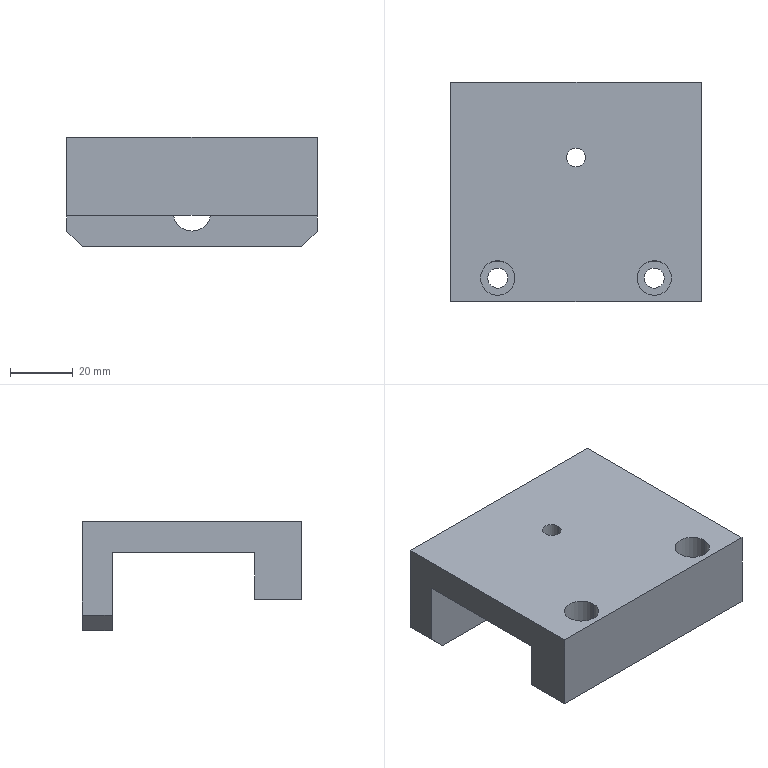Part | SolidWorks | features ICE 5, Chamfer 1, Extrusion 1, HoleWzd 1 | 1 solid | 26 faces | box 80 x 70 x 35 mm | volume 87735 mm3 | plane 14 | cylinder 12 | commonest cylinder face diameters 6.4 x4 11 x4 6 x2 12 x2
STEP:
#1=CARTESIAN_POINT('',(40.,60.5,7.));
#2=VERTEX_POINT('',#1);
#3=CARTESIAN_POINT('',(40.,60.5,-5.));
#4=VERTEX_POINT('',#3);
#5=CARTESIAN_POINT('',(40.,60.5,1.));
#6=DIRECTION('',(0.,-1.,0.));
#7=DIRECTION('',(0.,0.,1.));
#8=AXIS2_PLACEMENT_3D('',#5,#6,#7);
#9=CIRCLE('',#8,6.);
#10=EDGE_CURVE('',#2,#4,#9,.T.);
#11=ORIENTED_EDGE('',*,*,#10,.T.);
#12=CARTESIAN_POINT('',(40.,70.,-5.));
#13=VERTEX_POINT('',#12);
#14=CARTESIAN_POINT('',(40.,43.529,-5.));
#15=DIRECTION('',(0.,1.,0.));
#16=VECTOR('',#15,1000.);
#17=LINE('',#14,#16);
#18=EDGE_CURVE('',#4,#13,#17,.T.);
#19=ORIENTED_EDGE('',*,*,#18,.T.);
#20=CARTESIAN_POINT('',(40.,70.,7.));
#21=VERTEX_POINT('',#20);
#22=CARTESIAN_POINT('',(40.,70.,1.));
#23=DIRECTION('',(0.,1.,0.));
#24=DIRECTION('',(0.,0.,1.));
#25=AXIS2_PLACEMENT_3D('',#22,#23,#24);
#26=CIRCLE('',#25,6.);
#27=EDGE_CURVE('',#13,#21,#26,.T.);
#28=ORIENTED_EDGE('',*,*,#27,.T.);
#29=CARTESIAN_POINT('',(40.,43.529,7.));
#30=DIRECTION('',(0.,1.,0.));
#31=VECTOR('',#30,1000.);
#32=LINE('',#29,#31);
#33=EDGE_CURVE('',#2,#21,#32,.T.);
#34=ORIENTED_EDGE('',*,*,#33,.F.);
#35=EDGE_LOOP('',(#11,#19,#28,#34));
#36=FACE_OUTER_BOUND('',#35,.T.);
#37=CARTESIAN_POINT('',(40.,43.529,1.));
#38=DIRECTION('',(0.,1.,0.));
#39=DIRECTION('',(0.,0.,1.));
#40=AXIS2_PLACEMENT_3D('',#37,#38,#39);
#41=CYLINDRICAL_SURFACE('',#40,6.);
#42=ADVANCED_FACE('',(#36),#41,.F.);
#43=CARTESIAN_POINT('',(37.,46.,15.));
#44=VERTEX_POINT('',#43);
#45=CARTESIAN_POINT('',(43.,46.,15.));
#46=VERTEX_POINT('',#45);
#47=CARTESIAN_POINT('',(40.,46.,15.));
#48=DIRECTION('',(0.,0.,1.));
#49=DIRECTION('',(1.,0.,0.));
#50=AXIS2_PLACEMENT_3D('',#47,#48,#49);
#51=CIRCLE('',#50,3.);
#52=EDGE_CURVE('',#44,#46,#51,.T.);
#53=ORIENTED_EDGE('',*,*,#52,.F.);
#54=CARTESIAN_POINT('',(37.,46.,25.));
#55=VERTEX_POINT('',#54);
#56=CARTESIAN_POINT('',(37.,46.,15.));
#57=DIRECTION('',(0.,0.,1.));
#58=VECTOR('',#57,1000.);
#59=LINE('',#56,#58);
#60=EDGE_CURVE('',#44,#55,#59,.T.);
#61=ORIENTED_EDGE('',*,*,#60,.T.);
#62=CARTESIAN_POINT('',(43.,46.,25.));
#63=VERTEX_POINT('',#62);
#64=CARTESIAN_POINT('',(40.,46.,25.));
#65=DIRECTION('',(0.,0.,1.));
#66=DIRECTION('',(1.,0.,0.));
#67=AXIS2_PLACEMENT_3D('',#64,#65,#66);
#68=CIRCLE('',#67,3.);
#69=EDGE_CURVE('',#55,#63,#68,.T.);
#70=ORIENTED_EDGE('',*,*,#69,.T.);
#71=CARTESIAN_POINT('',(43.,46.,15.));
#72=DIRECTION('',(0.,0.,1.));
#73=VECTOR('',#72,1000.);
#74=LINE('',#71,#73);
#75=EDGE_CURVE('',#46,#63,#74,.T.);
#76=ORIENTED_EDGE('',*,*,#75,.F.);
#77=EDGE_LOOP('',(#53,#61,#70,#76));
#78=FACE_OUTER_BOUND('',#77,.T.);
#79=CARTESIAN_POINT('',(40.,46.,15.));
#80=DIRECTION('',(0.,0.,1.));
#81=DIRECTION('',(1.,0.,0.));
#82=AXIS2_PLACEMENT_3D('',#79,#80,#81);
#83=CYLINDRICAL_SURFACE('',#82,3.);
#84=ADVANCED_FACE('',(#78),#83,.F.);
#85=CARTESIAN_POINT('',(9.5,7.5,8.6));
#86=VERTEX_POINT('',#85);
#87=CARTESIAN_POINT('',(20.5,7.5,8.6));
#88=VERTEX_POINT('',#87);
#89=CARTESIAN_POINT('',(15.,7.5,8.6));
#90=DIRECTION('',(0.,0.,1.));
#91=DIRECTION('',(1.,0.,0.));
#92=AXIS2_PLACEMENT_3D('',#89,#90,#91);
#93=CIRCLE('',#92,5.5);
#94=EDGE_CURVE('',#86,#88,#93,.T.);
#95=ORIENTED_EDGE('',*,*,#94,.F.);
#96=CARTESIAN_POINT('',(9.5,7.5,25.));
#97=VERTEX_POINT('',#96);
#98=CARTESIAN_POINT('',(9.5,7.5,25.));
#99=DIRECTION('',(0.,0.,1.));
#100=VECTOR('',#99,1000.);
#101=LINE('',#98,#100);
#102=EDGE_CURVE('',#86,#97,#101,.T.);
#103=ORIENTED_EDGE('',*,*,#102,.T.);
#104=CARTESIAN_POINT('',(20.5,7.5,25.));
#105=VERTEX_POINT('',#104);
#106=CARTESIAN_POINT('',(15.,7.5,25.));
#107=DIRECTION('',(0.,0.,1.));
#108=DIRECTION('',(1.,0.,0.));
#109=AXIS2_PLACEMENT_3D('',#106,#107,#108);
#110=CIRCLE('',#109,5.5);
#111=EDGE_CURVE('',#97,#105,#110,.T.);
#112=ORIENTED_EDGE('',*,*,#111,.T.);
#113=CARTESIAN_POINT('',(20.5,7.5,25.));
#114=DIRECTION('',(0.,0.,1.));
#115=VECTOR('',#114,1000.);
#116=LINE('',#113,#115);
#117=EDGE_CURVE('',#88,#105,#116,.T.);
#118=ORIENTED_EDGE('',*,*,#117,.F.);
#119=EDGE_LOOP('',(#95,#103,#112,#118));
#120=FACE_OUTER_BOUND('',#119,.T.);
#121=CARTESIAN_POINT('',(15.,7.5,25.));
#122=DIRECTION('',(0.,0.,1.));
#123=DIRECTION('',(1.,0.,0.));
#124=AXIS2_PLACEMENT_3D('',#121,#122,#123);
#125=CYLINDRICAL_SURFACE('',#124,5.5);
#126=ADVANCED_FACE('',(#120),#125,.F.);
#127=CARTESIAN_POINT('',(59.5,7.5,8.6));
#128=VERTEX_POINT('',#127);
#129=CARTESIAN_POINT('',(70.5,7.5,8.6));
#130=VERTEX_POINT('',#129);
#131=CARTESIAN_POINT('',(65.,7.5,8.6));
#132=DIRECTION('',(0.,0.,1.));
#133=DIRECTION('',(1.,0.,0.));
#134=AXIS2_PLACEMENT_3D('',#131,#132,#133);
#135=CIRCLE('',#134,5.5);
#136=EDGE_CURVE('',#128,#130,#135,.T.);
#137=ORIENTED_EDGE('',*,*,#136,.F.);
#138=CARTESIAN_POINT('',(59.5,7.5,25.));
#139=VERTEX_POINT('',#138);
#140=CARTESIAN_POINT('',(59.5,7.5,25.));
#141=DIRECTION('',(0.,0.,1.));
#142=VECTOR('',#141,1000.);
#143=LINE('',#140,#142);
#144=EDGE_CURVE('',#128,#139,#143,.T.);
#145=ORIENTED_EDGE('',*,*,#144,.T.);
#146=CARTESIAN_POINT('',(70.5,7.5,25.));
#147=VERTEX_POINT('',#146);
#148=CARTESIAN_POINT('',(65.,7.5,25.));
#149=DIRECTION('',(0.,0.,1.));
#150=DIRECTION('',(1.,0.,0.));
#151=AXIS2_PLACEMENT_3D('',#148,#149,#150);
#152=CIRCLE('',#151,5.5);
#153=EDGE_CURVE('',#139,#147,#152,.T.);
#154=ORIENTED_EDGE('',*,*,#153,.T.);
#155=CARTESIAN_POINT('',(70.5,7.5,25.));
#156=DIRECTION('',(0.,0.,1.));
#157=VECTOR('',#156,1000.);
#158=LINE('',#155,#157);
#159=EDGE_CURVE('',#130,#147,#158,.T.);
#160=ORIENTED_EDGE('',*,*,#159,.F.);
#161=EDGE_LOOP('',(#137,#145,#154,#160));
#162=FACE_OUTER_BOUND('',#161,.T.);
#163=CARTESIAN_POINT('',(65.,7.5,25.));
#164=DIRECTION('',(0.,0.,1.));
#165=DIRECTION('',(1.,0.,0.));
#166=AXIS2_PLACEMENT_3D('',#163,#164,#165);
#167=CYLINDRICAL_SURFACE('',#166,5.5);
#168=ADVANCED_FACE('',(#162),#167,.F.);
#169=CARTESIAN_POINT('',(11.8,7.5,0.));
#170=VERTEX_POINT('',#169);
#171=CARTESIAN_POINT('',(18.2,7.5,0.));
#172=VERTEX_POINT('',#171);
#173=CARTESIAN_POINT('',(15.,7.5,0.));
#174=DIRECTION('',(0.,0.,1.));
#175=DIRECTION('',(1.,0.,0.));
#176=AXIS2_PLACEMENT_3D('',#173,#174,#175);
#177=CIRCLE('',#176,3.2);
#178=EDGE_CURVE('',#170,#172,#177,.T.);
#179=ORIENTED_EDGE('',*,*,#178,.F.);
#180=CARTESIAN_POINT('',(11.8,7.5,8.6));
#181=VERTEX_POINT('',#180);
#182=CARTESIAN_POINT('',(11.8,7.5,25.));
#183=DIRECTION('',(0.,0.,1.));
#184=VECTOR('',#183,1000.);
#185=LINE('',#182,#184);
#186=EDGE_CURVE('',#170,#181,#185,.T.);
#187=ORIENTED_EDGE('',*,*,#186,.T.);
#188=CARTESIAN_POINT('',(18.2,7.5,8.6));
#189=VERTEX_POINT('',#188);
#190=CARTESIAN_POINT('',(15.,7.5,8.6));
#191=DIRECTION('',(0.,0.,-1.));
#192=DIRECTION('',(1.,0.,0.));
#193=AXIS2_PLACEMENT_3D('',#190,#191,#192);
#194=CIRCLE('',#193,3.2);
#195=EDGE_CURVE('',#189,#181,#194,.T.);
#196=ORIENTED_EDGE('',*,*,#195,.F.);
#197=CARTESIAN_POINT('',(18.2,7.5,25.));
#198=DIRECTION('',(0.,0.,1.));
#199=VECTOR('',#198,1000.);
#200=LINE('',#197,#199);
#201=EDGE_CURVE('',#172,#189,#200,.T.);
#202=ORIENTED_EDGE('',*,*,#201,.F.);
#203=EDGE_LOOP('',(#179,#187,#196,#202));
#204=FACE_OUTER_BOUND('',#203,.T.);
#205=CARTESIAN_POINT('',(15.,7.5,25.));
#206=DIRECTION('',(0.,0.,1.));
#207=DIRECTION('',(1.,0.,0.));
#208=AXIS2_PLACEMENT_3D('',#205,#206,#207);
#209=CYLINDRICAL_SURFACE('',#208,3.2);
#210=ADVANCED_FACE('',(#204),#209,.F.);
#211=CARTESIAN_POINT('',(61.8,7.5,0.));
#212=VERTEX_POINT('',#211);
#213=CARTESIAN_POINT('',(68.2,7.5,0.));
#214=VERTEX_POINT('',#213);
#215=CARTESIAN_POINT('',(65.,7.5,0.));
#216=DIRECTION('',(0.,0.,1.));
#217=DIRECTION('',(1.,0.,0.));
#218=AXIS2_PLACEMENT_3D('',#215,#216,#217);
#219=CIRCLE('',#218,3.2);
#220=EDGE_CURVE('',#212,#214,#219,.T.);
#221=ORIENTED_EDGE('',*,*,#220,.F.);
#222=CARTESIAN_POINT('',(61.8,7.5,8.6));
#223=VERTEX_POINT('',#222);
#224=CARTESIAN_POINT('',(61.8,7.5,25.));
#225=DIRECTION('',(0.,0.,1.));
#226=VECTOR('',#225,1000.);
#227=LINE('',#224,#226);
#228=EDGE_CURVE('',#212,#223,#227,.T.);
#229=ORIENTED_EDGE('',*,*,#228,.T.);
#230=CARTESIAN_POINT('',(68.2,7.5,8.6));
#231=VERTEX_POINT('',#230);
#232=CARTESIAN_POINT('',(65.,7.5,8.6));
#233=DIRECTION('',(0.,0.,-1.));
#234=DIRECTION('',(1.,0.,0.));
#235=AXIS2_PLACEMENT_3D('',#232,#233,#234);
#236=CIRCLE('',#235,3.2);
#237=EDGE_CURVE('',#231,#223,#236,.T.);
#238=ORIENTED_EDGE('',*,*,#237,.F.);
#239=CARTESIAN_POINT('',(68.2,7.5,25.));
#240=DIRECTION('',(0.,0.,1.));
#241=VECTOR('',#240,1000.);
#242=LINE('',#239,#241);
#243=EDGE_CURVE('',#214,#231,#242,.T.);
#244=ORIENTED_EDGE('',*,*,#243,.F.);
#245=EDGE_LOOP('',(#221,#229,#238,#244));
#246=FACE_OUTER_BOUND('',#245,.T.);
#247=CARTESIAN_POINT('',(65.,7.5,25.));
#248=DIRECTION('',(0.,0.,1.));
#249=DIRECTION('',(1.,0.,0.));
#250=AXIS2_PLACEMENT_3D('',#247,#248,#249);
#251=CYLINDRICAL_SURFACE('',#250,3.2);
#252=ADVANCED_FACE('',(#246),#251,.F.);
#253=ORIENTED_EDGE('',*,*,#228,.F.);
#254=CARTESIAN_POINT('',(65.,7.5,0.));
#255=DIRECTION('',(0.,0.,1.));
#256=DIRECTION('',(1.,0.,0.));
#257=AXIS2_PLACEMENT_3D('',#254,#255,#256);
#258=CIRCLE('',#257,3.2);
#259=EDGE_CURVE('',#214,#212,#258,.T.);
#260=ORIENTED_EDGE('',*,*,#259,.F.);
#261=ORIENTED_EDGE('',*,*,#243,.T.);
#262=CARTESIAN_POINT('',(65.,7.5,8.6));
#263=DIRECTION('',(0.,0.,-1.));
#264=DIRECTION('',(1.,0.,0.));
#265=AXIS2_PLACEMENT_3D('',#262,#263,#264);
#266=CIRCLE('',#265,3.2);
#267=EDGE_CURVE('',#223,#231,#266,.T.);
#268=ORIENTED_EDGE('',*,*,#267,.F.);
#269=EDGE_LOOP('',(#253,#260,#261,#268));
#270=FACE_OUTER_BOUND('',#269,.T.);
#271=CARTESIAN_POINT('',(65.,7.5,25.));
#272=DIRECTION('',(0.,0.,1.));
#273=DIRECTION('',(1.,0.,0.));
#274=AXIS2_PLACEMENT_3D('',#271,#272,#273);
#275=CYLINDRICAL_SURFACE('',#274,3.2);
#276=ADVANCED_FACE('',(#270),#275,.F.);
#277=ORIENTED_EDGE('',*,*,#186,.F.);
#278=CARTESIAN_POINT('',(15.,7.5,0.));
#279=DIRECTION('',(0.,0.,1.));
#280=DIRECTION('',(1.,0.,0.));
#281=AXIS2_PLACEMENT_3D('',#278,#279,#280);
#282=CIRCLE('',#281,3.2);
#283=EDGE_CURVE('',#172,#170,#282,.T.);
#284=ORIENTED_EDGE('',*,*,#283,.F.);
#285=ORIENTED_EDGE('',*,*,#201,.T.);
#286=CARTESIAN_POINT('',(15.,7.5,8.6));
#287=DIRECTION('',(0.,0.,-1.));
#288=DIRECTION('',(1.,0.,0.));
#289=AXIS2_PLACEMENT_3D('',#286,#287,#288);
#290=CIRCLE('',#289,3.2);
#291=EDGE_CURVE('',#181,#189,#290,.T.);
#292=ORIENTED_EDGE('',*,*,#291,.F.);
#293=EDGE_LOOP('',(#277,#284,#285,#292));
#294=FACE_OUTER_BOUND('',#293,.T.);
#295=CARTESIAN_POINT('',(15.,7.5,25.));
#296=DIRECTION('',(0.,0.,1.));
#297=DIRECTION('',(1.,0.,0.));
#298=AXIS2_PLACEMENT_3D('',#295,#296,#297);
#299=CYLINDRICAL_SURFACE('',#298,3.2);
#300=ADVANCED_FACE('',(#294),#299,.F.);
#301=CARTESIAN_POINT('',(0.,70.,25.));
#302=VERTEX_POINT('',#301);
#303=CARTESIAN_POINT('',(0.,70.,-5.));
#304=VERTEX_POINT('',#303);
#305=CARTESIAN_POINT('',(0.,70.,25.));
#306=DIRECTION('',(0.,0.,-1.));
#307=VECTOR('',#306,1000.);
#308=LINE('',#305,#307);
#309=EDGE_CURVE('',#302,#304,#308,.T.);
#310=ORIENTED_EDGE('',*,*,#309,.T.);
#311=CARTESIAN_POINT('',(0.,60.5,-5.));
#312=VERTEX_POINT('',#311);
#313=CARTESIAN_POINT('',(0.,60.5,-5.));
#314=DIRECTION('',(0.,-1.,0.));
#315=VECTOR('',#314,1000.);
#316=LINE('',#313,#315);
#317=EDGE_CURVE('',#304,#312,#316,.T.);
#318=ORIENTED_EDGE('',*,*,#317,.T.);
#319=CARTESIAN_POINT('',(0.,60.5,15.));
#320=VERTEX_POINT('',#319);
#321=CARTESIAN_POINT('',(0.,60.5,25.));
#322=DIRECTION('',(0.,0.,1.));
#323=VECTOR('',#322,1000.);
#324=LINE('',#321,#323);
#325=EDGE_CURVE('',#312,#320,#324,.T.);
#326=ORIENTED_EDGE('',*,*,#325,.T.);
#327=CARTESIAN_POINT('',(0.,15.,15.));
#328=VERTEX_POINT('',#327);
#329=CARTESIAN_POINT('',(0.,0.,15.));
#330=DIRECTION('',(0.,-1.,0.));
#331=VECTOR('',#330,1000.);
#332=LINE('',#329,#331);
#333=EDGE_CURVE('',#320,#328,#332,.T.);
#334=ORIENTED_EDGE('',*,*,#333,.T.);
#335=CARTESIAN_POINT('',(0.,15.,0.));
#336=VERTEX_POINT('',#335);
#337=CARTESIAN_POINT('',(0.,15.,25.));
#338=DIRECTION('',(0.,0.,-1.));
#339=VECTOR('',#338,1000.);
#340=LINE('',#337,#339);
#341=EDGE_CURVE('',#328,#336,#340,.T.);
#342=ORIENTED_EDGE('',*,*,#341,.T.);
#343=CARTESIAN_POINT('',(0.,0.,0.));
#344=VERTEX_POINT('',#343);
#345=CARTESIAN_POINT('',(0.,0.,0.));
#346=DIRECTION('',(0.,-1.,0.));
#347=VECTOR('',#346,1000.);
#348=LINE('',#345,#347);
#349=EDGE_CURVE('',#336,#344,#348,.T.);
#350=ORIENTED_EDGE('',*,*,#349,.T.);
#351=CARTESIAN_POINT('',(0.,0.,25.));
#352=VERTEX_POINT('',#351);
#353=CARTESIAN_POINT('',(0.,0.,25.));
#354=DIRECTION('',(0.,0.,-1.));
#355=VECTOR('',#354,1000.);
#356=LINE('',#353,#355);
#357=EDGE_CURVE('',#352,#344,#356,.T.);
#358=ORIENTED_EDGE('',*,*,#357,.F.);
#359=CARTESIAN_POINT('',(0.,0.,25.));
#360=DIRECTION('',(0.,-1.,0.));
#361=VECTOR('',#360,1000.);
#362=LINE('',#359,#361);
#363=EDGE_CURVE('',#302,#352,#362,.T.);
#364=ORIENTED_EDGE('',*,*,#363,.F.);
#365=EDGE_LOOP('',(#310,#318,#326,#334,#342,#350,#358,#364));
#366=FACE_OUTER_BOUND('',#365,.T.);
#367=CARTESIAN_POINT('',(0.,0.,25.));
#368=DIRECTION('',(1.,0.,0.));
#369=DIRECTION('',(0.,1.,0.));
#370=AXIS2_PLACEMENT_3D('',#367,#368,#369);
#371=PLANE('',#370);
#372=ADVANCED_FACE('',(#366),#371,.F.);
#373=CARTESIAN_POINT('',(80.,0.,0.));
#374=VERTEX_POINT('',#373);
#375=CARTESIAN_POINT('',(0.,0.,0.));
#376=DIRECTION('',(1.,0.,0.));
#377=VECTOR('',#376,1000.);
#378=LINE('',#375,#377);
#379=EDGE_CURVE('',#344,#374,#378,.T.);
#380=ORIENTED_EDGE('',*,*,#379,.T.);
#381=CARTESIAN_POINT('',(80.,0.,25.));
#382=VERTEX_POINT('',#381);
#383=CARTESIAN_POINT('',(80.,0.,25.));
#384=DIRECTION('',(0.,0.,-1.));
#385=VECTOR('',#384,1000.);
#386=LINE('',#383,#385);
#387=EDGE_CURVE('',#382,#374,#386,.T.);
#388=ORIENTED_EDGE('',*,*,#387,.F.);
#389=CARTESIAN_POINT('',(0.,0.,25.));
#390=DIRECTION('',(1.,0.,0.));
#391=VECTOR('',#390,1000.);
#392=LINE('',#389,#391);
#393=EDGE_CURVE('',#352,#382,#392,.T.);
#394=ORIENTED_EDGE('',*,*,#393,.F.);
#395=ORIENTED_EDGE('',*,*,#357,.T.);
#396=EDGE_LOOP('',(#380,#388,#394,#395));
#397=FACE_OUTER_BOUND('',#396,.T.);
#398=CARTESIAN_POINT('',(0.,0.,25.));
#399=DIRECTION('',(0.,1.,0.));
#400=DIRECTION('',(0.,0.,1.));
#401=AXIS2_PLACEMENT_3D('',#398,#399,#400);
#402=PLANE('',#401);
#403=ADVANCED_FACE('',(#397),#402,.F.);
#404=CARTESIAN_POINT('',(80.,60.5,-5.));
#405=VERTEX_POINT('',#404);
#406=CARTESIAN_POINT('',(80.,60.5,15.));
#407=VERTEX_POINT('',#406);
#408=CARTESIAN_POINT('',(80.,60.5,15.));
#409=DIRECTION('',(0.,0.,1.));
#410=VECTOR('',#409,1000.);
#411=LINE('',#408,#410);
#412=EDGE_CURVE('',#405,#407,#411,.T.);
#413=ORIENTED_EDGE('',*,*,#412,.F.);
#414=CARTESIAN_POINT('',(80.,70.,-5.));
#415=VERTEX_POINT('',#414);
#416=CARTESIAN_POINT('',(80.,70.,-5.));
#417=DIRECTION('',(0.,1.,0.));
#418=VECTOR('',#417,1000.);
#419=LINE('',#416,#418);
#420=EDGE_CURVE('',#405,#415,#419,.T.);
#421=ORIENTED_EDGE('',*,*,#420,.T.);
#422=CARTESIAN_POINT('',(80.,70.,25.));
#423=VERTEX_POINT('',#422);
#424=CARTESIAN_POINT('',(80.,70.,25.));
#425=DIRECTION('',(0.,0.,-1.));
#426=VECTOR('',#425,1000.);
#427=LINE('',#424,#426);
#428=EDGE_CURVE('',#423,#415,#427,.T.);
#429=ORIENTED_EDGE('',*,*,#428,.F.);
#430=CARTESIAN_POINT('',(80.,0.,25.));
#431=DIRECTION('',(0.,1.,0.));
#432=VECTOR('',#431,1000.);
#433=LINE('',#430,#432);
#434=EDGE_CURVE('',#382,#423,#433,.T.);
#435=ORIENTED_EDGE('',*,*,#434,.F.);
#436=ORIENTED_EDGE('',*,*,#387,.T.);
#437=CARTESIAN_POINT('',(80.,15.,0.));
#438=VERTEX_POINT('',#437);
#439=CARTESIAN_POINT('',(80.,0.,0.));
#440=DIRECTION('',(0.,1.,0.));
#441=VECTOR('',#440,1000.);
#442=LINE('',#439,#441);
#443=EDGE_CURVE('',#374,#438,#442,.T.);
#444=ORIENTED_EDGE('',*,*,#443,.T.);
#445=CARTESIAN_POINT('',(80.,15.,15.));
#446=VERTEX_POINT('',#445);
#447=CARTESIAN_POINT('',(80.,15.,15.));
#448=DIRECTION('',(0.,0.,-1.));
#449=VECTOR('',#448,1000.);
#450=LINE('',#447,#449);
#451=EDGE_CURVE('',#446,#438,#450,.T.);
#452=ORIENTED_EDGE('',*,*,#451,.F.);
#453=CARTESIAN_POINT('',(80.,60.5,15.));
#454=DIRECTION('',(0.,-1.,0.));
#455=VECTOR('',#454,1000.);
#456=LINE('',#453,#455);
#457=EDGE_CURVE('',#407,#446,#456,.T.);
#458=ORIENTED_EDGE('',*,*,#457,.F.);
#459=EDGE_LOOP('',(#413,#421,#429,#435,#436,#444,#452,#458));
#460=FACE_OUTER_BOUND('',#459,.T.);
#461=CARTESIAN_POINT('',(80.,0.,25.));
#462=DIRECTION('',(-1.,0.,0.));
#463=DIRECTION('',(0.,-1.,0.));
#464=AXIS2_PLACEMENT_3D('',#461,#462,#463);
#465=PLANE('',#464);
#466=ADVANCED_FACE('',(#460),#465,.F.);
#467=CARTESIAN_POINT('',(40.,70.,1.));
#468=DIRECTION('',(0.,1.,0.));
#469=DIRECTION('',(0.,0.,1.));
#470=AXIS2_PLACEMENT_3D('',#467,#468,#469);
#471=CIRCLE('',#470,6.);
#472=EDGE_CURVE('',#21,#13,#471,.T.);
#473=ORIENTED_EDGE('',*,*,#472,.F.);
#474=ORIENTED_EDGE('',*,*,#27,.F.);
#475=EDGE_LOOP('',(#473,#474));
#476=FACE_BOUND('',#475,.T.);
#477=CARTESIAN_POINT('',(5.,70.,-10.));
#478=VERTEX_POINT('',#477);
#479=CARTESIAN_POINT('',(75.,70.,-10.));
#480=VERTEX_POINT('',#479);
#481=CARTESIAN_POINT('',(0.,70.,-10.));
#482=DIRECTION('',(1.,0.,0.));
#483=VECTOR('',#482,1000.);
#484=LINE('',#481,#483);
#485=EDGE_CURVE('',#478,#480,#484,.T.);
#486=ORIENTED_EDGE('',*,*,#485,.F.);
#487=CARTESIAN_POINT('',(5.,70.,-10.));
#488=DIRECTION('',(-0.7071,0.,0.7071));
#489=VECTOR('',#488,1000.);
#490=LINE('',#487,#489);
#491=EDGE_CURVE('',#478,#304,#490,.T.);
#492=ORIENTED_EDGE('',*,*,#491,.T.);
#493=ORIENTED_EDGE('',*,*,#309,.F.);
#494=CARTESIAN_POINT('',(0.,70.,25.));
#495=DIRECTION('',(-1.,0.,0.));
#496=VECTOR('',#495,1000.);
#497=LINE('',#494,#496);
#498=EDGE_CURVE('',#423,#302,#497,.T.);
#499=ORIENTED_EDGE('',*,*,#498,.F.);
#500=ORIENTED_EDGE('',*,*,#428,.T.);
#501=CARTESIAN_POINT('',(75.,70.,-10.));
#502=DIRECTION('',(-0.7071,0.,-0.7071));
#503=VECTOR('',#502,1000.);
#504=LINE('',#501,#503);
#505=EDGE_CURVE('',#415,#480,#504,.T.);
#506=ORIENTED_EDGE('',*,*,#505,.T.);
#507=EDGE_LOOP('',(#486,#492,#493,#499,#500,#506));
#508=FACE_OUTER_BOUND('',#507,.T.);
#509=CARTESIAN_POINT('',(0.,70.,25.));
#510=DIRECTION('',(0.,-1.,0.));
#511=DIRECTION('',(0.,0.,-1.));
#512=AXIS2_PLACEMENT_3D('',#509,#510,#511);
#513=PLANE('',#512);
#514=ADVANCED_FACE('',(#476,#508),#513,.F.);
#515=CARTESIAN_POINT('',(40.,46.,25.));
#516=DIRECTION('',(0.,0.,1.));
#517=DIRECTION('',(1.,0.,0.));
#518=AXIS2_PLACEMENT_3D('',#515,#516,#517);
#519=CIRCLE('',#518,3.);
#520=EDGE_CURVE('',#63,#55,#519,.T.);
#521=ORIENTED_EDGE('',*,*,#520,.F.);
#522=ORIENTED_EDGE('',*,*,#69,.F.);
#523=EDGE_LOOP('',(#521,#522));
#524=FACE_BOUND('',#523,.T.);
#525=CARTESIAN_POINT('',(15.,7.5,25.));
#526=DIRECTION('',(0.,0.,1.));
#527=DIRECTION('',(1.,0.,0.));
#528=AXIS2_PLACEMENT_3D('',#525,#526,#527);
#529=CIRCLE('',#528,5.5);
#530=EDGE_CURVE('',#105,#97,#529,.T.);
#531=ORIENTED_EDGE('',*,*,#530,.F.);
#532=ORIENTED_EDGE('',*,*,#111,.F.);
#533=EDGE_LOOP('',(#531,#532));
#534=FACE_BOUND('',#533,.T.);
#535=CARTESIAN_POINT('',(65.,7.5,25.));
#536=DIRECTION('',(0.,0.,1.));
#537=DIRECTION('',(1.,0.,0.));
#538=AXIS2_PLACEMENT_3D('',#535,#536,#537);
#539=CIRCLE('',#538,5.5);
#540=EDGE_CURVE('',#147,#139,#539,.T.);
#541=ORIENTED_EDGE('',*,*,#540,.F.);
#542=ORIENTED_EDGE('',*,*,#153,.F.);
#543=EDGE_LOOP('',(#541,#542));
#544=FACE_BOUND('',#543,.T.);
#545=ORIENTED_EDGE('',*,*,#363,.T.);
#546=ORIENTED_EDGE('',*,*,#393,.T.);
#547=ORIENTED_EDGE('',*,*,#434,.T.);
#548=ORIENTED_EDGE('',*,*,#498,.T.);
#549=EDGE_LOOP('',(#545,#546,#547,#548));
#550=FACE_OUTER_BOUND('',#549,.T.);
#551=CARTESIAN_POINT('',(0.,0.,25.));
#552=DIRECTION('',(0.,0.,-1.));
#553=DIRECTION('',(-1.,0.,0.));
#554=AXIS2_PLACEMENT_3D('',#551,#552,#553);
#555=PLANE('',#554);
#556=ADVANCED_FACE('',(#524,#534,#544,#550),#555,.F.);
#557=ORIENTED_EDGE('',*,*,#283,.T.);
#558=ORIENTED_EDGE('',*,*,#178,.T.);
#559=EDGE_LOOP('',(#557,#558));
#560=FACE_BOUND('',#559,.T.);
#561=ORIENTED_EDGE('',*,*,#259,.T.);
#562=ORIENTED_EDGE('',*,*,#220,.T.);
#563=EDGE_LOOP('',(#561,#562));
#564=FACE_BOUND('',#563,.T.);
#565=CARTESIAN_POINT('',(0.,15.,0.));
#566=DIRECTION('',(-1.,0.,0.));
#567=VECTOR('',#566,1000.);
#568=LINE('',#565,#567);
#569=EDGE_CURVE('',#438,#336,#568,.T.);
#570=ORIENTED_EDGE('',*,*,#569,.F.);
#571=ORIENTED_EDGE('',*,*,#443,.F.);
#572=ORIENTED_EDGE('',*,*,#379,.F.);
#573=ORIENTED_EDGE('',*,*,#349,.F.);
#574=EDGE_LOOP('',(#570,#571,#572,#573));
#575=FACE_OUTER_BOUND('',#574,.T.);
#576=CARTESIAN_POINT('',(0.,0.,0.));
#577=DIRECTION('',(0.,0.,-1.));
#578=DIRECTION('',(-1.,0.,0.));
#579=AXIS2_PLACEMENT_3D('',#576,#577,#578);
#580=PLANE('',#579);
#581=ADVANCED_FACE('',(#560,#564,#575),#580,.T.);
#582=CARTESIAN_POINT('',(40.,46.,15.));
#583=DIRECTION('',(0.,0.,1.));
#584=DIRECTION('',(1.,0.,0.));
#585=AXIS2_PLACEMENT_3D('',#582,#583,#584);
#586=CIRCLE('',#585,3.);
#587=EDGE_CURVE('',#46,#44,#586,.T.);
#588=ORIENTED_EDGE('',*,*,#587,.T.);
#589=ORIENTED_EDGE('',*,*,#52,.T.);
#590=EDGE_LOOP('',(#588,#589));
#591=FACE_BOUND('',#590,.T.);
#592=CARTESIAN_POINT('',(-29.,60.5,15.));
#593=DIRECTION('',(1.,0.,0.));
#594=VECTOR('',#593,1000.);
#595=LINE('',#592,#594);
#596=EDGE_CURVE('',#320,#407,#595,.T.);
#597=ORIENTED_EDGE('',*,*,#596,.T.);
#598=ORIENTED_EDGE('',*,*,#457,.T.);
#599=CARTESIAN_POINT('',(-29.,15.,15.));
#600=DIRECTION('',(1.,0.,0.));
#601=VECTOR('',#600,1000.);
#602=LINE('',#599,#601);
#603=EDGE_CURVE('',#328,#446,#602,.T.);
#604=ORIENTED_EDGE('',*,*,#603,.F.);
#605=ORIENTED_EDGE('',*,*,#333,.F.);
#606=EDGE_LOOP('',(#597,#598,#604,#605));
#607=FACE_OUTER_BOUND('',#606,.T.);
#608=CARTESIAN_POINT('',(-29.,60.5,15.));
#609=DIRECTION('',(0.,0.,1.));
#610=DIRECTION('',(0.,-1.,0.));
#611=AXIS2_PLACEMENT_3D('',#608,#609,#610);
#612=PLANE('',#611);
#613=ADVANCED_FACE('',(#591,#607),#612,.F.);
#614=ORIENTED_EDGE('',*,*,#10,.F.);
#615=CARTESIAN_POINT('',(40.,60.5,1.));
#616=DIRECTION('',(0.,-1.,0.));
#617=DIRECTION('',(0.,0.,1.));
#618=AXIS2_PLACEMENT_3D('',#615,#616,#617);
#619=CIRCLE('',#618,6.);
#620=EDGE_CURVE('',#4,#2,#619,.T.);
#621=ORIENTED_EDGE('',*,*,#620,.F.);
#622=EDGE_LOOP('',(#614,#621));
#623=FACE_BOUND('',#622,.T.);
#624=ORIENTED_EDGE('',*,*,#325,.F.);
#625=CARTESIAN_POINT('',(5.,60.5,-10.));
#626=VERTEX_POINT('',#625);
#627=CARTESIAN_POINT('',(5.,60.5,-10.));
#628=DIRECTION('',(0.7071,0.,-0.7071));
#629=VECTOR('',#628,1000.);
#630=LINE('',#627,#629);
#631=EDGE_CURVE('',#312,#626,#630,.T.);
#632=ORIENTED_EDGE('',*,*,#631,.T.);
#633=CARTESIAN_POINT('',(75.,60.5,-10.));
#634=VERTEX_POINT('',#633);
#635=CARTESIAN_POINT('',(80.,60.5,-10.));
#636=DIRECTION('',(-1.,0.,0.));
#637=VECTOR('',#636,1000.);
#638=LINE('',#635,#637);
#639=EDGE_CURVE('',#634,#626,#638,.T.);
#640=ORIENTED_EDGE('',*,*,#639,.F.);
#641=CARTESIAN_POINT('',(75.,60.5,-10.));
#642=DIRECTION('',(0.7071,0.,0.7071));
#643=VECTOR('',#642,1000.);
#644=LINE('',#641,#643);
#645=EDGE_CURVE('',#634,#405,#644,.T.);
#646=ORIENTED_EDGE('',*,*,#645,.T.);
#647=ORIENTED_EDGE('',*,*,#412,.T.);
#648=ORIENTED_EDGE('',*,*,#596,.F.);
#649=EDGE_LOOP('',(#624,#632,#640,#646,#647,#648));
#650=FACE_OUTER_BOUND('',#649,.T.);
#651=CARTESIAN_POINT('',(-29.,60.5,15.));
#652=DIRECTION('',(0.,1.,0.));
#653=DIRECTION('',(0.,0.,1.));
#654=AXIS2_PLACEMENT_3D('',#651,#652,#653);
#655=PLANE('',#654);
#656=ADVANCED_FACE('',(#623,#650),#655,.F.);
#657=ORIENTED_EDGE('',*,*,#603,.T.);
#658=ORIENTED_EDGE('',*,*,#451,.T.);
#659=ORIENTED_EDGE('',*,*,#569,.T.);
#660=ORIENTED_EDGE('',*,*,#341,.F.);
#661=EDGE_LOOP('',(#657,#658,#659,#660));
#662=FACE_OUTER_BOUND('',#661,.T.);
#663=CARTESIAN_POINT('',(-29.,15.,15.));
#664=DIRECTION('',(0.,-1.,0.));
#665=DIRECTION('',(0.,0.,-1.));
#666=AXIS2_PLACEMENT_3D('',#663,#664,#665);
#667=PLANE('',#666);
#668=ADVANCED_FACE('',(#662),#667,.F.);
#669=ORIENTED_EDGE('',*,*,#144,.F.);
#670=CARTESIAN_POINT('',(65.,7.5,8.6));
#671=DIRECTION('',(0.,0.,1.));
#672=DIRECTION('',(1.,0.,0.));
#673=AXIS2_PLACEMENT_3D('',#670,#671,#672);
#674=CIRCLE('',#673,5.5);
#675=EDGE_CURVE('',#130,#128,#674,.T.);
#676=ORIENTED_EDGE('',*,*,#675,.F.);
#677=ORIENTED_EDGE('',*,*,#159,.T.);
#678=ORIENTED_EDGE('',*,*,#540,.T.);
#679=EDGE_LOOP('',(#669,#676,#677,#678));
#680=FACE_OUTER_BOUND('',#679,.T.);
#681=CARTESIAN_POINT('',(65.,7.5,25.));
#682=DIRECTION('',(0.,0.,1.));
#683=DIRECTION('',(1.,0.,0.));
#684=AXIS2_PLACEMENT_3D('',#681,#682,#683);
#685=CYLINDRICAL_SURFACE('',#684,5.5);
#686=ADVANCED_FACE('',(#680),#685,.F.);
#687=ORIENTED_EDGE('',*,*,#102,.F.);
#688=CARTESIAN_POINT('',(15.,7.5,8.6));
#689=DIRECTION('',(0.,0.,1.));
#690=DIRECTION('',(1.,0.,0.));
#691=AXIS2_PLACEMENT_3D('',#688,#689,#690);
#692=CIRCLE('',#691,5.5);
#693=EDGE_CURVE('',#88,#86,#692,.T.);
#694=ORIENTED_EDGE('',*,*,#693,.F.);
#695=ORIENTED_EDGE('',*,*,#117,.T.);
#696=ORIENTED_EDGE('',*,*,#530,.T.);
#697=EDGE_LOOP('',(#687,#694,#695,#696));
#698=FACE_OUTER_BOUND('',#697,.T.);
#699=CARTESIAN_POINT('',(15.,7.5,25.));
#700=DIRECTION('',(0.,0.,1.));
#701=DIRECTION('',(1.,0.,0.));
#702=AXIS2_PLACEMENT_3D('',#699,#700,#701);
#703=CYLINDRICAL_SURFACE('',#702,5.5);
#704=ADVANCED_FACE('',(#698),#703,.F.);
#705=ORIENTED_EDGE('',*,*,#693,.T.);
#706=ORIENTED_EDGE('',*,*,#94,.T.);
#707=EDGE_LOOP('',(#705,#706));
#708=FACE_OUTER_BOUND('',#707,.T.);
#709=ORIENTED_EDGE('',*,*,#195,.T.);
#710=ORIENTED_EDGE('',*,*,#291,.T.);
#711=EDGE_LOOP('',(#709,#710));
#712=FACE_BOUND('',#711,.T.);
#713=CARTESIAN_POINT('',(15.,7.5,8.6));
#714=DIRECTION('',(0.,0.,1.));
#715=DIRECTION('',(1.,0.,0.));
#716=AXIS2_PLACEMENT_3D('',#713,#714,#715);
#717=PLANE('',#716);
#718=ADVANCED_FACE('',(#708,#712),#717,.T.);
#719=ORIENTED_EDGE('',*,*,#675,.T.);
#720=ORIENTED_EDGE('',*,*,#136,.T.);
#721=EDGE_LOOP('',(#719,#720));
#722=FACE_OUTER_BOUND('',#721,.T.);
#723=ORIENTED_EDGE('',*,*,#237,.T.);
#724=ORIENTED_EDGE('',*,*,#267,.T.);
#725=EDGE_LOOP('',(#723,#724));
#726=FACE_BOUND('',#725,.T.);
#727=CARTESIAN_POINT('',(65.,7.5,8.6));
#728=DIRECTION('',(0.,0.,1.));
#729=DIRECTION('',(1.,0.,0.));
#730=AXIS2_PLACEMENT_3D('',#727,#728,#729);
#731=PLANE('',#730);
#732=ADVANCED_FACE('',(#722,#726),#731,.T.);
#733=ORIENTED_EDGE('',*,*,#60,.F.);
#734=ORIENTED_EDGE('',*,*,#587,.F.);
#735=ORIENTED_EDGE('',*,*,#75,.T.);
#736=ORIENTED_EDGE('',*,*,#520,.T.);
#737=EDGE_LOOP('',(#733,#734,#735,#736));
#738=FACE_OUTER_BOUND('',#737,.T.);
#739=CARTESIAN_POINT('',(40.,46.,15.));
#740=DIRECTION('',(0.,0.,1.));
#741=DIRECTION('',(1.,0.,0.));
#742=AXIS2_PLACEMENT_3D('',#739,#740,#741);
#743=CYLINDRICAL_SURFACE('',#742,3.);
#744=ADVANCED_FACE('',(#738),#743,.F.);
#745=ORIENTED_EDGE('',*,*,#639,.T.);
#746=CARTESIAN_POINT('',(5.,70.,-10.));
#747=DIRECTION('',(0.,1.,0.));
#748=VECTOR('',#747,1000.);
#749=LINE('',#746,#748);
#750=EDGE_CURVE('',#626,#478,#749,.T.);
#751=ORIENTED_EDGE('',*,*,#750,.T.);
#752=ORIENTED_EDGE('',*,*,#485,.T.);
#753=CARTESIAN_POINT('',(75.,60.5,-10.));
#754=DIRECTION('',(0.,-1.,0.));
#755=VECTOR('',#754,1000.);
#756=LINE('',#753,#755);
#757=EDGE_CURVE('',#480,#634,#756,.T.);
#758=ORIENTED_EDGE('',*,*,#757,.T.);
#759=EDGE_LOOP('',(#745,#751,#752,#758));
#760=FACE_OUTER_BOUND('',#759,.T.);
#761=CARTESIAN_POINT('',(0.,0.,-10.));
#762=DIRECTION('',(0.,0.,-1.));
#763=DIRECTION('',(-1.,0.,0.));
#764=AXIS2_PLACEMENT_3D('',#761,#762,#763);
#765=PLANE('',#764);
#766=ADVANCED_FACE('',(#760),#765,.T.);
#767=ORIENTED_EDGE('',*,*,#18,.F.);
#768=ORIENTED_EDGE('',*,*,#620,.T.);
#769=ORIENTED_EDGE('',*,*,#33,.T.);
#770=ORIENTED_EDGE('',*,*,#472,.T.);
#771=EDGE_LOOP('',(#767,#768,#769,#770));
#772=FACE_OUTER_BOUND('',#771,.T.);
#773=CARTESIAN_POINT('',(40.,43.529,1.));
#774=DIRECTION('',(0.,1.,0.));
#775=DIRECTION('',(0.,0.,1.));
#776=AXIS2_PLACEMENT_3D('',#773,#774,#775);
#777=CYLINDRICAL_SURFACE('',#776,6.);
#778=ADVANCED_FACE('',(#772),#777,.F.);
#779=ORIENTED_EDGE('',*,*,#631,.F.);
#780=ORIENTED_EDGE('',*,*,#317,.F.);
#781=ORIENTED_EDGE('',*,*,#491,.F.);
#782=ORIENTED_EDGE('',*,*,#750,.F.);
#783=EDGE_LOOP('',(#779,#780,#781,#782));
#784=FACE_OUTER_BOUND('',#783,.T.);
#785=CARTESIAN_POINT('',(5.,0.,-10.));
#786=DIRECTION('',(-0.7071,0.,-0.7071));
#787=DIRECTION('',(0.,-1.,0.));
#788=AXIS2_PLACEMENT_3D('',#785,#786,#787);
#789=PLANE('',#788);
#790=ADVANCED_FACE('',(#784),#789,.T.);
#791=ORIENTED_EDGE('',*,*,#505,.F.);
#792=ORIENTED_EDGE('',*,*,#420,.F.);
#793=ORIENTED_EDGE('',*,*,#645,.F.);
#794=ORIENTED_EDGE('',*,*,#757,.F.);
#795=EDGE_LOOP('',(#791,#792,#793,#794));
#796=FACE_OUTER_BOUND('',#795,.T.);
#797=CARTESIAN_POINT('',(75.,0.,-10.));
#798=DIRECTION('',(0.7071,0.,-0.7071));
#799=DIRECTION('',(0.,1.,0.));
#800=AXIS2_PLACEMENT_3D('',#797,#798,#799);
#801=PLANE('',#800);
#802=ADVANCED_FACE('',(#796),#801,.T.);
#803=CLOSED_SHELL('',(#42,#84,#126,#168,#210,#252,#276,#300,#372,#403,#466,#514,#556,#581,#613,#656,#668,#686,#704,#718,#732,#744,#766,#778,#790,#802));
#804=MANIFOLD_SOLID_BREP('',#803);
#805=CARTESIAN_POINT('',(0.,0.,0.));
#806=DIRECTION('',(0.,0.,1.));
#807=DIRECTION('',(1.,0.,0.));
#808=AXIS2_PLACEMENT_3D('',#805,#806,#807);
#809=(LENGTH_UNIT()NAMED_UNIT(*)SI_UNIT(.MILLI.,.METRE.));
#810=UNCERTAINTY_MEASURE_WITH_UNIT(LENGTH_MEASURE(0.00001),#809,'','');
#811=(NAMED_UNIT(*)PLANE_ANGLE_UNIT()SI_UNIT($,.RADIAN.));
#812=(NAMED_UNIT(*)SI_UNIT($,.STERADIAN.)SOLID_ANGLE_UNIT());
#813=(GEOMETRIC_REPRESENTATION_CONTEXT(3)GLOBAL_UNCERTAINTY_ASSIGNED_CONTEXT((#810))GLOBAL_UNIT_ASSIGNED_CONTEXT((#809,#811,#812))REPRESENTATION_CONTEXT('',''));
#814=ADVANCED_BREP_SHAPE_REPRESENTATION('',(#804,#808),#813);